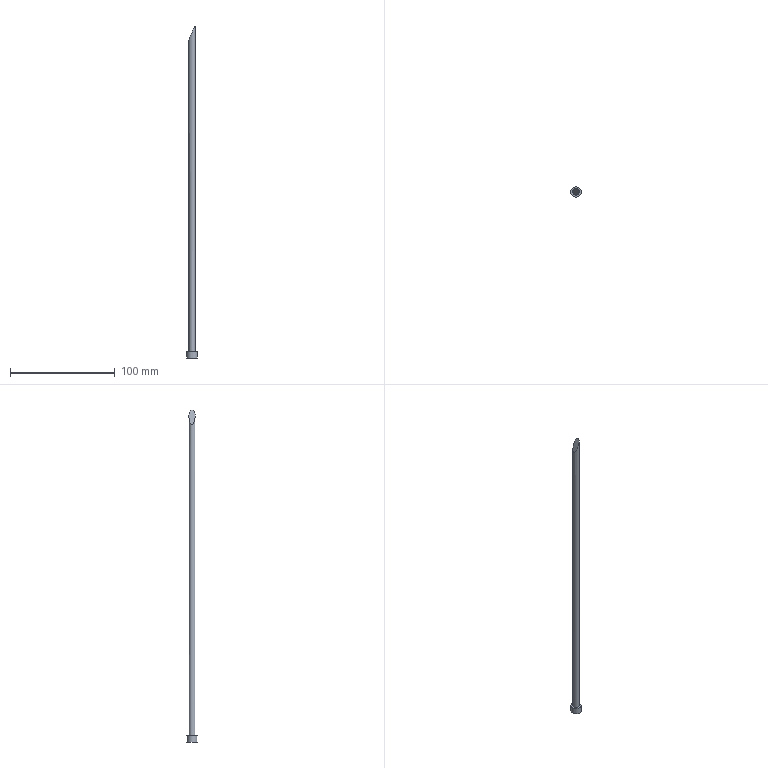Part | NX | features solid 2 | 1 solid | 5 faces | box 10 x 10 x 317.079 mm | volume 9086 mm3 | cylinder 2 | plane 2 | spline 1 | commonest cylinder face diameters 6 x1 10 x1
STEP:
#1=CARTESIAN_POINT('',(-56.,31.,-339.5));
#2=VERTEX_POINT('',#1);
#3=CARTESIAN_POINT('',(-59.,31.,-339.5));
#4=DIRECTION('',(0.,0.,-1.));
#5=DIRECTION('',(1.,0.,0.));
#6=AXIS2_PLACEMENT_3D('',#3,#4,#5);
#7=CIRCLE('',#6,3.);
#8=EDGE_CURVE('',#2,#2,#7,.T.);
#9=ORIENTED_EDGE('',*,*,#8,.F.);
#10=EDGE_LOOP('',(#9));
#11=FACE_BOUND('',#10,.T.);
#12=CARTESIAN_POINT('',(-56.01,31.245,-28.447));
#13=VERTEX_POINT('',#12);
#14=CARTESIAN_POINT('',(-56.22,32.228,-28.893));
#15=CARTESIAN_POINT('',(-55.943,31.279,-28.321));
#16=CARTESIAN_POINT('',(-56.067,30.126,-28.502));
#17=CARTESIAN_POINT('',(-56.455,29.356,-29.211));
#18=CARTESIAN_POINT('',(-56.898,28.829,-30.057));
#19=CARTESIAN_POINT('',(-57.51,28.351,-31.27));
#20=CARTESIAN_POINT('',(-58.282,28.039,-32.882));
#21=CARTESIAN_POINT('',(-59.161,27.964,-34.832));
#22=CARTESIAN_POINT('',(-60.005,28.131,-36.826));
#23=CARTESIAN_POINT('',(-60.654,28.464,-38.454));
#24=CARTESIAN_POINT('',(-61.14,28.877,-39.73));
#25=CARTESIAN_POINT('',(-61.49,29.294,-40.681));
#26=CARTESIAN_POINT('',(-61.799,29.843,-41.553));
#27=CARTESIAN_POINT('',(-62.055,30.718,-42.316));
#28=CARTESIAN_POINT('',(-61.926,31.876,-42.021));
#29=CARTESIAN_POINT('',(-61.603,32.528,-41.168));
#30=CARTESIAN_POINT('',(-61.259,33.001,-40.273));
#31=CARTESIAN_POINT('',(-60.758,33.468,-38.99));
#32=CARTESIAN_POINT('',(-60.105,33.832,-37.374));
#33=CARTESIAN_POINT('',(-59.274,34.028,-35.407));
#34=CARTESIAN_POINT('',(-58.395,33.984,-33.428));
#35=CARTESIAN_POINT('',(-57.501,33.664,-31.506));
#36=CARTESIAN_POINT('',(-56.743,33.064,-29.949));
#37=CARTESIAN_POINT('',(-56.22,32.228,-28.893));
#38=CARTESIAN_POINT('',(-55.943,31.279,-28.321));
#39=CARTESIAN_POINT('',(-56.067,30.126,-28.502));
#40=B_SPLINE_CURVE_WITH_KNOTS('',3,(#14,#15,#16,#17,#18,#19,#20,#21,#22,#23,#24,#25,#26,#27,#28,#29,#30,#31,#32,#33,#34,#35,#36,#37,#38,#39),.UNSPECIFIED.,.T.,.F.,(1,1,1,1,1,1,1,1,1,1,1,1,1,1,1,1,1,1,1,1,1,1,1,1,1,1,1,1,1,1),(-0.004355,-0.002177,-0.001089,0.,0.001089,0.002177,0.003266,0.004355,0.006532,0.008709,0.01089,0.01306,0.01415,0.01524,0.01633,0.01742,0.01851,0.0196,0.02068,0.02177,0.02395,0.02613,0.0283,0.03048,0.03266,0.03375,0.03484,0.03593,0.03701,0.0381),.UNSPECIFIED.);
#41=EDGE_CURVE('',#13,#13,#40,.T.);
#42=ORIENTED_EDGE('',*,*,#41,.T.);
#43=EDGE_LOOP('',(#42));
#44=FACE_BOUND('',#43,.T.);
#45=CARTESIAN_POINT('',(-59.,31.,-345.5));
#46=DIRECTION('',(0.,0.,1.));
#47=DIRECTION('',(1.,0.,0.));
#48=AXIS2_PLACEMENT_3D('',#45,#46,#47);
#49=CYLINDRICAL_SURFACE('',#48,3.);
#50=ADVANCED_FACE('',(#11,#44),#49,.T.);
#51=ORIENTED_EDGE('',*,*,#8,.T.);
#52=EDGE_LOOP('',(#51));
#53=FACE_BOUND('',#52,.T.);
#54=CARTESIAN_POINT('',(-54.,31.,-339.5));
#55=VERTEX_POINT('',#54);
#56=CARTESIAN_POINT('',(-59.,31.,-339.5));
#57=DIRECTION('',(0.,0.,1.));
#58=DIRECTION('',(1.,0.,0.));
#59=AXIS2_PLACEMENT_3D('',#56,#57,#58);
#60=CIRCLE('',#59,5.);
#61=EDGE_CURVE('',#55,#55,#60,.T.);
#62=ORIENTED_EDGE('',*,*,#61,.T.);
#63=EDGE_LOOP('',(#62));
#64=FACE_BOUND('',#63,.T.);
#65=CARTESIAN_POINT('',(-59.,31.,-339.5));
#66=DIRECTION('',(0.,0.,1.));
#67=DIRECTION('',(1.,0.,0.));
#68=AXIS2_PLACEMENT_3D('',#65,#66,#67);
#69=PLANE('',#68);
#70=ADVANCED_FACE('',(#53,#64),#69,.T.);
#71=CARTESIAN_POINT('',(-54.,31.,-345.5));
#72=VERTEX_POINT('',#71);
#73=CARTESIAN_POINT('',(-59.,31.,-345.5));
#74=DIRECTION('',(0.,0.,-1.));
#75=DIRECTION('',(1.,0.,0.));
#76=AXIS2_PLACEMENT_3D('',#73,#74,#75);
#77=CIRCLE('',#76,5.);
#78=EDGE_CURVE('',#72,#72,#77,.T.);
#79=ORIENTED_EDGE('',*,*,#78,.T.);
#80=EDGE_LOOP('',(#79));
#81=FACE_BOUND('',#80,.T.);
#82=CARTESIAN_POINT('',(-59.,31.,-345.5));
#83=DIRECTION('',(0.,0.,-1.));
#84=DIRECTION('',(-1.,0.,0.));
#85=AXIS2_PLACEMENT_3D('',#82,#83,#84);
#86=PLANE('',#85);
#87=ADVANCED_FACE('',(#81),#86,.T.);
#88=ORIENTED_EDGE('',*,*,#61,.F.);
#89=EDGE_LOOP('',(#88));
#90=FACE_BOUND('',#89,.T.);
#91=ORIENTED_EDGE('',*,*,#78,.F.);
#92=EDGE_LOOP('',(#91));
#93=FACE_BOUND('',#92,.T.);
#94=CARTESIAN_POINT('',(-59.,31.,-345.5));
#95=DIRECTION('',(0.,0.,1.));
#96=DIRECTION('',(1.,0.,0.));
#97=AXIS2_PLACEMENT_3D('',#94,#95,#96);
#98=CYLINDRICAL_SURFACE('',#97,5.);
#99=ADVANCED_FACE('',(#90,#93),#98,.T.);
#100=ORIENTED_EDGE('',*,*,#41,.F.);
#101=EDGE_LOOP('',(#100));
#102=FACE_BOUND('',#101,.T.);
#103=CARTESIAN_POINT('',(-62.066,27.902,-42.189));
#104=CARTESIAN_POINT('',(-62.044,29.949,-42.241));
#105=CARTESIAN_POINT('',(-62.021,31.996,-42.293));
#106=CARTESIAN_POINT('',(-61.997,34.043,-42.346));
#107=CARTESIAN_POINT('',(-60.887,27.902,-38.884));
#108=CARTESIAN_POINT('',(-60.864,29.949,-38.936));
#109=CARTESIAN_POINT('',(-60.841,31.996,-38.988));
#110=CARTESIAN_POINT('',(-60.817,34.043,-39.041));
#111=CARTESIAN_POINT('',(-59.564,27.902,-35.634));
#112=CARTESIAN_POINT('',(-59.542,29.949,-35.686));
#113=CARTESIAN_POINT('',(-59.518,31.996,-35.738));
#114=CARTESIAN_POINT('',(-59.494,34.043,-35.792));
#115=CARTESIAN_POINT('',(-57.417,27.902,-31.039));
#116=CARTESIAN_POINT('',(-57.395,29.949,-31.091));
#117=CARTESIAN_POINT('',(-57.371,31.996,-31.144));
#118=CARTESIAN_POINT('',(-57.347,34.042,-31.197));
#119=CARTESIAN_POINT('',(-56.72,27.902,-29.635));
#120=CARTESIAN_POINT('',(-56.697,29.949,-29.687));
#121=CARTESIAN_POINT('',(-56.674,31.996,-29.74));
#122=CARTESIAN_POINT('',(-56.65,34.043,-29.793));
#123=CARTESIAN_POINT('',(-55.988,27.902,-28.249));
#124=CARTESIAN_POINT('',(-55.966,29.949,-28.301));
#125=CARTESIAN_POINT('',(-55.943,31.996,-28.354));
#126=CARTESIAN_POINT('',(-55.919,34.043,-28.407));
#127=B_SPLINE_SURFACE_WITH_KNOTS('',3,3,((#103,#104,#105,#106),(#107,#108,#109,#110),(#111,#112,#113,#114),(#115,#116,#117,#118),(#119,#120,#121,#122),(#123,#124,#125,#126)),.UNSPECIFIED.,.F.,.F.,.F.,(4,2,4),(4,4),(0.1967,0.25,0.2738),(0.08168,0.1983),.UNSPECIFIED.);
#128=ADVANCED_FACE('',(#102),#127,.T.);
#129=CLOSED_SHELL('',(#50,#70,#87,#99,#128));
#130=MANIFOLD_SOLID_BREP('',#129);
#131=(LENGTH_UNIT()NAMED_UNIT(*)SI_UNIT(.MILLI.,.METRE.));
#132=UNCERTAINTY_MEASURE_WITH_UNIT(LENGTH_MEASURE(0.0508),#131,'','');
#133=(NAMED_UNIT(*)PLANE_ANGLE_UNIT()SI_UNIT($,.RADIAN.));
#134=(NAMED_UNIT(*)SI_UNIT($,.STERADIAN.)SOLID_ANGLE_UNIT());
#135=(GEOMETRIC_REPRESENTATION_CONTEXT(3)GLOBAL_UNCERTAINTY_ASSIGNED_CONTEXT((#132))GLOBAL_UNIT_ASSIGNED_CONTEXT((#131,#133,#134))REPRESENTATION_CONTEXT('',''));
#136=ADVANCED_BREP_SHAPE_REPRESENTATION('',(#130),#135);